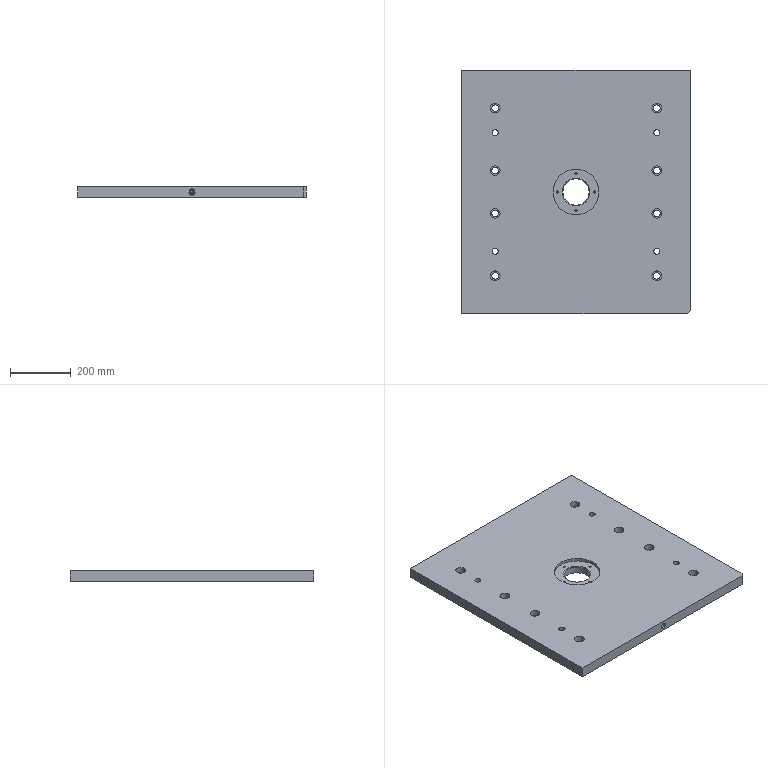Part | Creo | 1 solid | 122 faces | box 750 x 800 x 35 mm | volume 20428944 mm3 | cylinder 72 | plane 32 | cone 18 | commonest cylinder face diameters 20 x16 22 x16 32 x16 6.799 x8 6.8 x8 14 x4